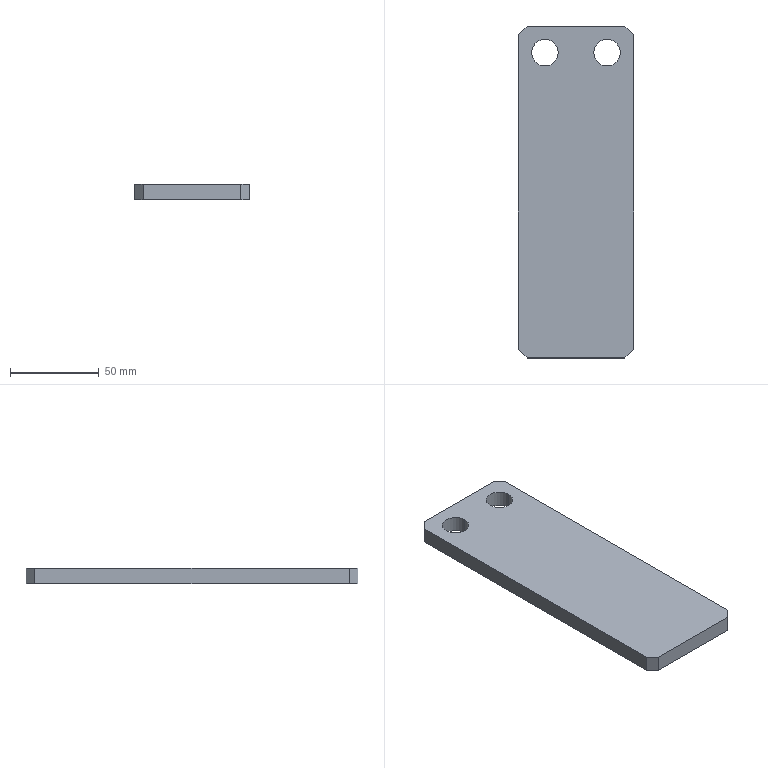Part | SolidWorks | features FlatPattern 1, SMBaseFlange 1, SheetMetal 1 | 1 solid | 14 faces | box 65 x 187 x 9 mm | volume 105764 mm3 | plane 10 | cylinder 4 | commonest cylinder face diameters 15 x4
STEP:
#1=CARTESIAN_POINT('',(42.5,172.,-9.));
#2=VERTEX_POINT('',#1);
#3=CARTESIAN_POINT('',(57.5,172.,-9.));
#4=VERTEX_POINT('',#3);
#5=CARTESIAN_POINT('',(50.,172.,-9.));
#6=DIRECTION('',(0.,0.,1.));
#7=DIRECTION('',(1.,0.,0.));
#8=AXIS2_PLACEMENT_3D('',#5,#6,#7);
#9=CIRCLE('',#8,7.5);
#10=EDGE_CURVE('',#2,#4,#9,.T.);
#11=ORIENTED_EDGE('',*,*,#10,.F.);
#12=CARTESIAN_POINT('',(42.5,172.,0.));
#13=VERTEX_POINT('',#12);
#14=CARTESIAN_POINT('',(42.5,172.,-9.));
#15=DIRECTION('',(0.,0.,1.));
#16=VECTOR('',#15,1000.);
#17=LINE('',#14,#16);
#18=EDGE_CURVE('',#2,#13,#17,.T.);
#19=ORIENTED_EDGE('',*,*,#18,.T.);
#20=CARTESIAN_POINT('',(57.5,172.,0.));
#21=VERTEX_POINT('',#20);
#22=CARTESIAN_POINT('',(50.,172.,0.));
#23=DIRECTION('',(0.,0.,1.));
#24=DIRECTION('',(1.,0.,0.));
#25=AXIS2_PLACEMENT_3D('',#22,#23,#24);
#26=CIRCLE('',#25,7.5);
#27=EDGE_CURVE('',#13,#21,#26,.T.);
#28=ORIENTED_EDGE('',*,*,#27,.T.);
#29=CARTESIAN_POINT('',(57.5,172.,-9.));
#30=DIRECTION('',(0.,0.,1.));
#31=VECTOR('',#30,1000.);
#32=LINE('',#29,#31);
#33=EDGE_CURVE('',#4,#21,#32,.T.);
#34=ORIENTED_EDGE('',*,*,#33,.F.);
#35=EDGE_LOOP('',(#11,#19,#28,#34));
#36=FACE_OUTER_BOUND('',#35,.T.);
#37=CARTESIAN_POINT('',(50.,172.,-9.));
#38=DIRECTION('',(0.,0.,1.));
#39=DIRECTION('',(1.,0.,0.));
#40=AXIS2_PLACEMENT_3D('',#37,#38,#39);
#41=CYLINDRICAL_SURFACE('',#40,7.5);
#42=ADVANCED_FACE('',(#36),#41,.F.);
#43=CARTESIAN_POINT('',(7.5,172.,-9.));
#44=VERTEX_POINT('',#43);
#45=CARTESIAN_POINT('',(22.5,172.,-9.));
#46=VERTEX_POINT('',#45);
#47=CARTESIAN_POINT('',(15.,172.,-9.));
#48=DIRECTION('',(0.,0.,1.));
#49=DIRECTION('',(1.,0.,0.));
#50=AXIS2_PLACEMENT_3D('',#47,#48,#49);
#51=CIRCLE('',#50,7.5);
#52=EDGE_CURVE('',#44,#46,#51,.T.);
#53=ORIENTED_EDGE('',*,*,#52,.F.);
#54=CARTESIAN_POINT('',(7.5,172.,0.));
#55=VERTEX_POINT('',#54);
#56=CARTESIAN_POINT('',(7.5,172.,-9.));
#57=DIRECTION('',(0.,0.,1.));
#58=VECTOR('',#57,1000.);
#59=LINE('',#56,#58);
#60=EDGE_CURVE('',#44,#55,#59,.T.);
#61=ORIENTED_EDGE('',*,*,#60,.T.);
#62=CARTESIAN_POINT('',(22.5,172.,0.));
#63=VERTEX_POINT('',#62);
#64=CARTESIAN_POINT('',(15.,172.,0.));
#65=DIRECTION('',(0.,0.,1.));
#66=DIRECTION('',(1.,0.,0.));
#67=AXIS2_PLACEMENT_3D('',#64,#65,#66);
#68=CIRCLE('',#67,7.5);
#69=EDGE_CURVE('',#55,#63,#68,.T.);
#70=ORIENTED_EDGE('',*,*,#69,.T.);
#71=CARTESIAN_POINT('',(22.5,172.,-9.));
#72=DIRECTION('',(0.,0.,1.));
#73=VECTOR('',#72,1000.);
#74=LINE('',#71,#73);
#75=EDGE_CURVE('',#46,#63,#74,.T.);
#76=ORIENTED_EDGE('',*,*,#75,.F.);
#77=EDGE_LOOP('',(#53,#61,#70,#76));
#78=FACE_OUTER_BOUND('',#77,.T.);
#79=CARTESIAN_POINT('',(15.,172.,-9.));
#80=DIRECTION('',(0.,0.,1.));
#81=DIRECTION('',(1.,0.,0.));
#82=AXIS2_PLACEMENT_3D('',#79,#80,#81);
#83=CYLINDRICAL_SURFACE('',#82,7.5);
#84=ADVANCED_FACE('',(#78),#83,.F.);
#85=CARTESIAN_POINT('',(0.,182.,0.));
#86=VERTEX_POINT('',#85);
#87=CARTESIAN_POINT('',(0.,5.,0.));
#88=VERTEX_POINT('',#87);
#89=CARTESIAN_POINT('',(0.,5.,0.));
#90=DIRECTION('',(0.,-1.,0.));
#91=VECTOR('',#90,1000.);
#92=LINE('',#89,#91);
#93=EDGE_CURVE('',#86,#88,#92,.T.);
#94=ORIENTED_EDGE('',*,*,#93,.F.);
#95=CARTESIAN_POINT('',(0.,182.,-9.));
#96=VERTEX_POINT('',#95);
#97=CARTESIAN_POINT('',(0.,182.,-9.));
#98=DIRECTION('',(0.,0.,1.));
#99=VECTOR('',#98,1000.);
#100=LINE('',#97,#99);
#101=EDGE_CURVE('',#96,#86,#100,.T.);
#102=ORIENTED_EDGE('',*,*,#101,.F.);
#103=CARTESIAN_POINT('',(0.,5.,-9.));
#104=VERTEX_POINT('',#103);
#105=CARTESIAN_POINT('',(0.,5.,-9.));
#106=DIRECTION('',(0.,-1.,0.));
#107=VECTOR('',#106,1000.);
#108=LINE('',#105,#107);
#109=EDGE_CURVE('',#96,#104,#108,.T.);
#110=ORIENTED_EDGE('',*,*,#109,.T.);
#111=CARTESIAN_POINT('',(0.,5.,-9.));
#112=DIRECTION('',(0.,0.,1.));
#113=VECTOR('',#112,1000.);
#114=LINE('',#111,#113);
#115=EDGE_CURVE('',#104,#88,#114,.T.);
#116=ORIENTED_EDGE('',*,*,#115,.T.);
#117=EDGE_LOOP('',(#94,#102,#110,#116));
#118=FACE_OUTER_BOUND('',#117,.T.);
#119=CARTESIAN_POINT('',(0.,5.,-9.));
#120=DIRECTION('',(-1.,0.,0.));
#121=DIRECTION('',(0.,0.,1.));
#122=AXIS2_PLACEMENT_3D('',#119,#120,#121);
#123=PLANE('',#122);
#124=ADVANCED_FACE('',(#118),#123,.T.);
#125=CARTESIAN_POINT('',(5.,187.,0.));
#126=VERTEX_POINT('',#125);
#127=CARTESIAN_POINT('',(0.,182.,0.));
#128=DIRECTION('',(-0.7071,-0.7071,0.));
#129=VECTOR('',#128,1000.);
#130=LINE('',#127,#129);
#131=EDGE_CURVE('',#126,#86,#130,.T.);
#132=ORIENTED_EDGE('',*,*,#131,.F.);
#133=CARTESIAN_POINT('',(5.,187.,-9.));
#134=VERTEX_POINT('',#133);
#135=CARTESIAN_POINT('',(5.,187.,-9.));
#136=DIRECTION('',(0.,0.,1.));
#137=VECTOR('',#136,1000.);
#138=LINE('',#135,#137);
#139=EDGE_CURVE('',#134,#126,#138,.T.);
#140=ORIENTED_EDGE('',*,*,#139,.F.);
#141=CARTESIAN_POINT('',(0.,182.,-9.));
#142=DIRECTION('',(-0.7071,-0.7071,0.));
#143=VECTOR('',#142,1000.);
#144=LINE('',#141,#143);
#145=EDGE_CURVE('',#134,#96,#144,.T.);
#146=ORIENTED_EDGE('',*,*,#145,.T.);
#147=ORIENTED_EDGE('',*,*,#101,.T.);
#148=EDGE_LOOP('',(#132,#140,#146,#147));
#149=FACE_OUTER_BOUND('',#148,.T.);
#150=CARTESIAN_POINT('',(0.,182.,-9.));
#151=DIRECTION('',(-0.7071,0.7071,0.));
#152=DIRECTION('',(-0.7071,-0.7071,0.));
#153=AXIS2_PLACEMENT_3D('',#150,#151,#152);
#154=PLANE('',#153);
#155=ADVANCED_FACE('',(#149),#154,.T.);
#156=CARTESIAN_POINT('',(60.,187.,0.));
#157=VERTEX_POINT('',#156);
#158=CARTESIAN_POINT('',(5.,187.,0.));
#159=DIRECTION('',(-1.,0.,0.));
#160=VECTOR('',#159,1000.);
#161=LINE('',#158,#160);
#162=EDGE_CURVE('',#157,#126,#161,.T.);
#163=ORIENTED_EDGE('',*,*,#162,.F.);
#164=CARTESIAN_POINT('',(60.,187.,-9.));
#165=VERTEX_POINT('',#164);
#166=CARTESIAN_POINT('',(60.,187.,-9.));
#167=DIRECTION('',(0.,0.,1.));
#168=VECTOR('',#167,1000.);
#169=LINE('',#166,#168);
#170=EDGE_CURVE('',#165,#157,#169,.T.);
#171=ORIENTED_EDGE('',*,*,#170,.F.);
#172=CARTESIAN_POINT('',(5.,187.,-9.));
#173=DIRECTION('',(-1.,0.,0.));
#174=VECTOR('',#173,1000.);
#175=LINE('',#172,#174);
#176=EDGE_CURVE('',#165,#134,#175,.T.);
#177=ORIENTED_EDGE('',*,*,#176,.T.);
#178=ORIENTED_EDGE('',*,*,#139,.T.);
#179=EDGE_LOOP('',(#163,#171,#177,#178));
#180=FACE_OUTER_BOUND('',#179,.T.);
#181=CARTESIAN_POINT('',(5.,187.,-9.));
#182=DIRECTION('',(0.,1.,0.));
#183=DIRECTION('',(0.,0.,1.));
#184=AXIS2_PLACEMENT_3D('',#181,#182,#183);
#185=PLANE('',#184);
#186=ADVANCED_FACE('',(#180),#185,.T.);
#187=CARTESIAN_POINT('',(65.,182.,0.));
#188=VERTEX_POINT('',#187);
#189=CARTESIAN_POINT('',(60.,187.,0.));
#190=DIRECTION('',(-0.7071,0.7071,0.));
#191=VECTOR('',#190,1000.);
#192=LINE('',#189,#191);
#193=EDGE_CURVE('',#188,#157,#192,.T.);
#194=ORIENTED_EDGE('',*,*,#193,.F.);
#195=CARTESIAN_POINT('',(65.,182.,-9.));
#196=VERTEX_POINT('',#195);
#197=CARTESIAN_POINT('',(65.,182.,-9.));
#198=DIRECTION('',(0.,0.,1.));
#199=VECTOR('',#198,1000.);
#200=LINE('',#197,#199);
#201=EDGE_CURVE('',#196,#188,#200,.T.);
#202=ORIENTED_EDGE('',*,*,#201,.F.);
#203=CARTESIAN_POINT('',(60.,187.,-9.));
#204=DIRECTION('',(-0.7071,0.7071,0.));
#205=VECTOR('',#204,1000.);
#206=LINE('',#203,#205);
#207=EDGE_CURVE('',#196,#165,#206,.T.);
#208=ORIENTED_EDGE('',*,*,#207,.T.);
#209=ORIENTED_EDGE('',*,*,#170,.T.);
#210=EDGE_LOOP('',(#194,#202,#208,#209));
#211=FACE_OUTER_BOUND('',#210,.T.);
#212=CARTESIAN_POINT('',(60.,187.,-9.));
#213=DIRECTION('',(0.7071,0.7071,0.));
#214=DIRECTION('',(-0.7071,0.7071,0.));
#215=AXIS2_PLACEMENT_3D('',#212,#213,#214);
#216=PLANE('',#215);
#217=ADVANCED_FACE('',(#211),#216,.T.);
#218=CARTESIAN_POINT('',(65.,5.,0.));
#219=VERTEX_POINT('',#218);
#220=CARTESIAN_POINT('',(65.,5.,0.));
#221=DIRECTION('',(0.,1.,0.));
#222=VECTOR('',#221,1000.);
#223=LINE('',#220,#222);
#224=EDGE_CURVE('',#219,#188,#223,.T.);
#225=ORIENTED_EDGE('',*,*,#224,.F.);
#226=CARTESIAN_POINT('',(65.,5.,-9.));
#227=VERTEX_POINT('',#226);
#228=CARTESIAN_POINT('',(65.,5.,-9.));
#229=DIRECTION('',(0.,0.,1.));
#230=VECTOR('',#229,1000.);
#231=LINE('',#228,#230);
#232=EDGE_CURVE('',#227,#219,#231,.T.);
#233=ORIENTED_EDGE('',*,*,#232,.F.);
#234=CARTESIAN_POINT('',(65.,5.,-9.));
#235=DIRECTION('',(0.,1.,0.));
#236=VECTOR('',#235,1000.);
#237=LINE('',#234,#236);
#238=EDGE_CURVE('',#227,#196,#237,.T.);
#239=ORIENTED_EDGE('',*,*,#238,.T.);
#240=ORIENTED_EDGE('',*,*,#201,.T.);
#241=EDGE_LOOP('',(#225,#233,#239,#240));
#242=FACE_OUTER_BOUND('',#241,.T.);
#243=CARTESIAN_POINT('',(65.,5.,-9.));
#244=DIRECTION('',(1.,0.,0.));
#245=DIRECTION('',(0.,0.,-1.));
#246=AXIS2_PLACEMENT_3D('',#243,#244,#245);
#247=PLANE('',#246);
#248=ADVANCED_FACE('',(#242),#247,.T.);
#249=CARTESIAN_POINT('',(60.,0.,0.));
#250=VERTEX_POINT('',#249);
#251=CARTESIAN_POINT('',(60.,0.,0.));
#252=DIRECTION('',(0.7071,0.7071,0.));
#253=VECTOR('',#252,1000.);
#254=LINE('',#251,#253);
#255=EDGE_CURVE('',#250,#219,#254,.T.);
#256=ORIENTED_EDGE('',*,*,#255,.F.);
#257=CARTESIAN_POINT('',(60.,0.,-9.));
#258=VERTEX_POINT('',#257);
#259=CARTESIAN_POINT('',(60.,0.,-9.));
#260=DIRECTION('',(0.,0.,1.));
#261=VECTOR('',#260,1000.);
#262=LINE('',#259,#261);
#263=EDGE_CURVE('',#258,#250,#262,.T.);
#264=ORIENTED_EDGE('',*,*,#263,.F.);
#265=CARTESIAN_POINT('',(60.,0.,-9.));
#266=DIRECTION('',(0.7071,0.7071,0.));
#267=VECTOR('',#266,1000.);
#268=LINE('',#265,#267);
#269=EDGE_CURVE('',#258,#227,#268,.T.);
#270=ORIENTED_EDGE('',*,*,#269,.T.);
#271=ORIENTED_EDGE('',*,*,#232,.T.);
#272=EDGE_LOOP('',(#256,#264,#270,#271));
#273=FACE_OUTER_BOUND('',#272,.T.);
#274=CARTESIAN_POINT('',(60.,0.,-9.));
#275=DIRECTION('',(0.7071,-0.7071,0.));
#276=DIRECTION('',(0.7071,0.7071,0.));
#277=AXIS2_PLACEMENT_3D('',#274,#275,#276);
#278=PLANE('',#277);
#279=ADVANCED_FACE('',(#273),#278,.T.);
#280=CARTESIAN_POINT('',(5.,0.,0.));
#281=VERTEX_POINT('',#280);
#282=CARTESIAN_POINT('',(5.,0.,0.));
#283=DIRECTION('',(1.,0.,0.));
#284=VECTOR('',#283,1000.);
#285=LINE('',#282,#284);
#286=EDGE_CURVE('',#281,#250,#285,.T.);
#287=ORIENTED_EDGE('',*,*,#286,.F.);
#288=CARTESIAN_POINT('',(5.,0.,-9.));
#289=VERTEX_POINT('',#288);
#290=CARTESIAN_POINT('',(5.,0.,-9.));
#291=DIRECTION('',(0.,0.,1.));
#292=VECTOR('',#291,1000.);
#293=LINE('',#290,#292);
#294=EDGE_CURVE('',#289,#281,#293,.T.);
#295=ORIENTED_EDGE('',*,*,#294,.F.);
#296=CARTESIAN_POINT('',(5.,0.,-9.));
#297=DIRECTION('',(1.,0.,0.));
#298=VECTOR('',#297,1000.);
#299=LINE('',#296,#298);
#300=EDGE_CURVE('',#289,#258,#299,.T.);
#301=ORIENTED_EDGE('',*,*,#300,.T.);
#302=ORIENTED_EDGE('',*,*,#263,.T.);
#303=EDGE_LOOP('',(#287,#295,#301,#302));
#304=FACE_OUTER_BOUND('',#303,.T.);
#305=CARTESIAN_POINT('',(5.,0.,-9.));
#306=DIRECTION('',(0.,-1.,0.));
#307=DIRECTION('',(0.,0.,-1.));
#308=AXIS2_PLACEMENT_3D('',#305,#306,#307);
#309=PLANE('',#308);
#310=ADVANCED_FACE('',(#304),#309,.T.);
#311=CARTESIAN_POINT('',(0.,5.,0.));
#312=DIRECTION('',(0.7071,-0.7071,0.));
#313=VECTOR('',#312,1000.);
#314=LINE('',#311,#313);
#315=EDGE_CURVE('',#88,#281,#314,.T.);
#316=ORIENTED_EDGE('',*,*,#315,.F.);
#317=ORIENTED_EDGE('',*,*,#115,.F.);
#318=CARTESIAN_POINT('',(0.,5.,-9.));
#319=DIRECTION('',(0.7071,-0.7071,0.));
#320=VECTOR('',#319,1000.);
#321=LINE('',#318,#320);
#322=EDGE_CURVE('',#104,#289,#321,.T.);
#323=ORIENTED_EDGE('',*,*,#322,.T.);
#324=ORIENTED_EDGE('',*,*,#294,.T.);
#325=EDGE_LOOP('',(#316,#317,#323,#324));
#326=FACE_OUTER_BOUND('',#325,.T.);
#327=CARTESIAN_POINT('',(0.,5.,-9.));
#328=DIRECTION('',(-0.7071,-0.7071,0.));
#329=DIRECTION('',(0.7071,-0.7071,0.));
#330=AXIS2_PLACEMENT_3D('',#327,#328,#329);
#331=PLANE('',#330);
#332=ADVANCED_FACE('',(#326),#331,.T.);
#333=CARTESIAN_POINT('',(50.,172.,-9.));
#334=DIRECTION('',(0.,0.,1.));
#335=DIRECTION('',(1.,0.,0.));
#336=AXIS2_PLACEMENT_3D('',#333,#334,#335);
#337=CIRCLE('',#336,7.5);
#338=EDGE_CURVE('',#4,#2,#337,.T.);
#339=ORIENTED_EDGE('',*,*,#338,.T.);
#340=ORIENTED_EDGE('',*,*,#10,.T.);
#341=EDGE_LOOP('',(#339,#340));
#342=FACE_BOUND('',#341,.T.);
#343=CARTESIAN_POINT('',(15.,172.,-9.));
#344=DIRECTION('',(0.,0.,1.));
#345=DIRECTION('',(1.,0.,0.));
#346=AXIS2_PLACEMENT_3D('',#343,#344,#345);
#347=CIRCLE('',#346,7.5);
#348=EDGE_CURVE('',#46,#44,#347,.T.);
#349=ORIENTED_EDGE('',*,*,#348,.T.);
#350=ORIENTED_EDGE('',*,*,#52,.T.);
#351=EDGE_LOOP('',(#349,#350));
#352=FACE_BOUND('',#351,.T.);
#353=ORIENTED_EDGE('',*,*,#109,.F.);
#354=ORIENTED_EDGE('',*,*,#145,.F.);
#355=ORIENTED_EDGE('',*,*,#176,.F.);
#356=ORIENTED_EDGE('',*,*,#207,.F.);
#357=ORIENTED_EDGE('',*,*,#238,.F.);
#358=ORIENTED_EDGE('',*,*,#269,.F.);
#359=ORIENTED_EDGE('',*,*,#300,.F.);
#360=ORIENTED_EDGE('',*,*,#322,.F.);
#361=EDGE_LOOP('',(#353,#354,#355,#356,#357,#358,#359,#360));
#362=FACE_OUTER_BOUND('',#361,.T.);
#363=CARTESIAN_POINT('',(0.,0.,-9.));
#364=DIRECTION('',(0.,0.,-1.));
#365=DIRECTION('',(-1.,0.,0.));
#366=AXIS2_PLACEMENT_3D('',#363,#364,#365);
#367=PLANE('',#366);
#368=ADVANCED_FACE('',(#342,#352,#362),#367,.T.);
#369=CARTESIAN_POINT('',(50.,172.,0.));
#370=DIRECTION('',(0.,0.,1.));
#371=DIRECTION('',(1.,0.,0.));
#372=AXIS2_PLACEMENT_3D('',#369,#370,#371);
#373=CIRCLE('',#372,7.5);
#374=EDGE_CURVE('',#21,#13,#373,.T.);
#375=ORIENTED_EDGE('',*,*,#374,.F.);
#376=ORIENTED_EDGE('',*,*,#27,.F.);
#377=EDGE_LOOP('',(#375,#376));
#378=FACE_BOUND('',#377,.T.);
#379=CARTESIAN_POINT('',(15.,172.,0.));
#380=DIRECTION('',(0.,0.,1.));
#381=DIRECTION('',(1.,0.,0.));
#382=AXIS2_PLACEMENT_3D('',#379,#380,#381);
#383=CIRCLE('',#382,7.5);
#384=EDGE_CURVE('',#63,#55,#383,.T.);
#385=ORIENTED_EDGE('',*,*,#384,.F.);
#386=ORIENTED_EDGE('',*,*,#69,.F.);
#387=EDGE_LOOP('',(#385,#386));
#388=FACE_BOUND('',#387,.T.);
#389=ORIENTED_EDGE('',*,*,#93,.T.);
#390=ORIENTED_EDGE('',*,*,#315,.T.);
#391=ORIENTED_EDGE('',*,*,#286,.T.);
#392=ORIENTED_EDGE('',*,*,#255,.T.);
#393=ORIENTED_EDGE('',*,*,#224,.T.);
#394=ORIENTED_EDGE('',*,*,#193,.T.);
#395=ORIENTED_EDGE('',*,*,#162,.T.);
#396=ORIENTED_EDGE('',*,*,#131,.T.);
#397=EDGE_LOOP('',(#389,#390,#391,#392,#393,#394,#395,#396));
#398=FACE_OUTER_BOUND('',#397,.T.);
#399=CARTESIAN_POINT('',(0.,0.,0.));
#400=DIRECTION('',(0.,0.,-1.));
#401=DIRECTION('',(-1.,0.,0.));
#402=AXIS2_PLACEMENT_3D('',#399,#400,#401);
#403=PLANE('',#402);
#404=ADVANCED_FACE('',(#378,#388,#398),#403,.F.);
#405=ORIENTED_EDGE('',*,*,#60,.F.);
#406=ORIENTED_EDGE('',*,*,#348,.F.);
#407=ORIENTED_EDGE('',*,*,#75,.T.);
#408=ORIENTED_EDGE('',*,*,#384,.T.);
#409=EDGE_LOOP('',(#405,#406,#407,#408));
#410=FACE_OUTER_BOUND('',#409,.T.);
#411=CARTESIAN_POINT('',(15.,172.,-9.));
#412=DIRECTION('',(0.,0.,1.));
#413=DIRECTION('',(1.,0.,0.));
#414=AXIS2_PLACEMENT_3D('',#411,#412,#413);
#415=CYLINDRICAL_SURFACE('',#414,7.5);
#416=ADVANCED_FACE('',(#410),#415,.F.);
#417=ORIENTED_EDGE('',*,*,#18,.F.);
#418=ORIENTED_EDGE('',*,*,#338,.F.);
#419=ORIENTED_EDGE('',*,*,#33,.T.);
#420=ORIENTED_EDGE('',*,*,#374,.T.);
#421=EDGE_LOOP('',(#417,#418,#419,#420));
#422=FACE_OUTER_BOUND('',#421,.T.);
#423=CARTESIAN_POINT('',(50.,172.,-9.));
#424=DIRECTION('',(0.,0.,1.));
#425=DIRECTION('',(1.,0.,0.));
#426=AXIS2_PLACEMENT_3D('',#423,#424,#425);
#427=CYLINDRICAL_SURFACE('',#426,7.5);
#428=ADVANCED_FACE('',(#422),#427,.F.);
#429=CLOSED_SHELL('',(#42,#84,#124,#155,#186,#217,#248,#279,#310,#332,#368,#404,#416,#428));
#430=MANIFOLD_SOLID_BREP('',#429);
#431=CARTESIAN_POINT('',(0.,0.,0.));
#432=DIRECTION('',(0.,0.,1.));
#433=DIRECTION('',(1.,0.,0.));
#434=AXIS2_PLACEMENT_3D('',#431,#432,#433);
#435=(LENGTH_UNIT()NAMED_UNIT(*)SI_UNIT(.MILLI.,.METRE.));
#436=UNCERTAINTY_MEASURE_WITH_UNIT(LENGTH_MEASURE(0.00001),#435,'','');
#437=(NAMED_UNIT(*)PLANE_ANGLE_UNIT()SI_UNIT($,.RADIAN.));
#438=(NAMED_UNIT(*)SI_UNIT($,.STERADIAN.)SOLID_ANGLE_UNIT());
#439=(GEOMETRIC_REPRESENTATION_CONTEXT(3)GLOBAL_UNCERTAINTY_ASSIGNED_CONTEXT((#436))GLOBAL_UNIT_ASSIGNED_CONTEXT((#435,#437,#438))REPRESENTATION_CONTEXT('',''));
#440=ADVANCED_BREP_SHAPE_REPRESENTATION('',(#430,#434),#439);